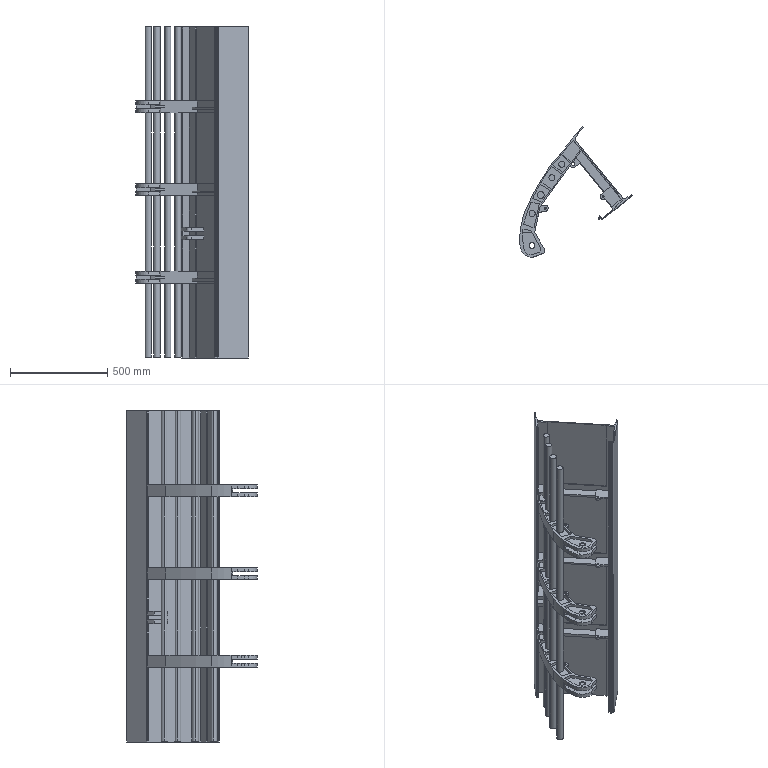Part | SolidWorks | features ICE 25, MirrorPattern 5, Extrusion 1 | 2 solids | 470 faces | box 578.108 x 670.148 x 1705 mm | volume 20388998 mm3 | plane 336 | cylinder 134 | commonest cylinder face diameters 30 x22 30.623 x16 1080 x11 10 x9 685.356 x9 765.342 x9